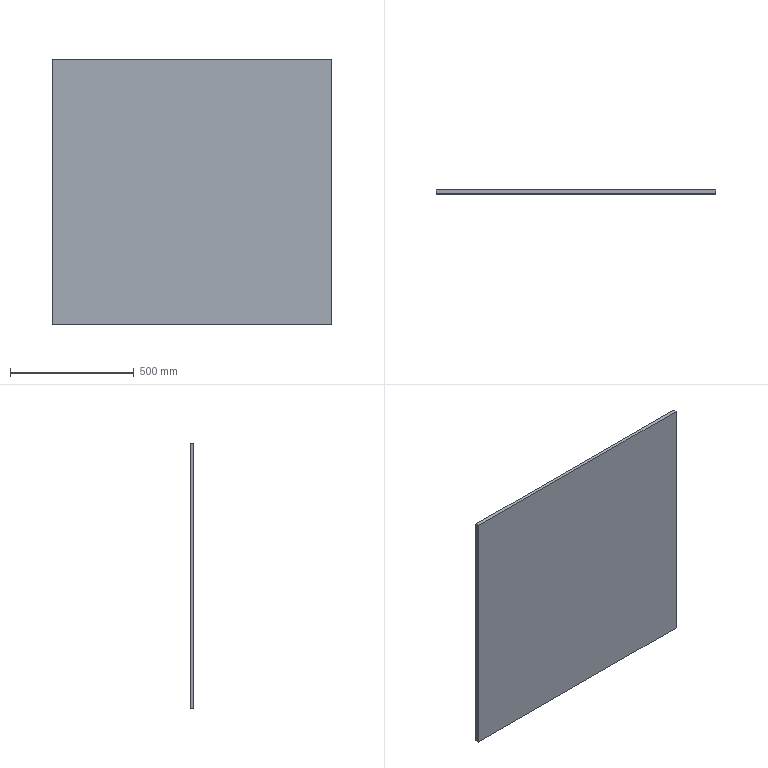Part | SolidWorks | features 3DProfileFeature 1, Extrusion 1, ICE 1 | 1 solid | 6 faces | box 1130 x 15 x 1072 mm | volume 18170400 mm3 | plane 6
STEP:
#1=CARTESIAN_POINT('',(565.,0.,536.));
#2=VERTEX_POINT('',#1);
#3=CARTESIAN_POINT('',(565.,0.,-536.));
#4=VERTEX_POINT('',#3);
#5=CARTESIAN_POINT('',(565.,0.,536.));
#6=DIRECTION('',(0.,0.,-1.));
#7=VECTOR('',#6,1000.);
#8=LINE('',#5,#7);
#9=EDGE_CURVE('',#2,#4,#8,.T.);
#10=ORIENTED_EDGE('',*,*,#9,.T.);
#11=CARTESIAN_POINT('',(565.,15.,-536.));
#12=VERTEX_POINT('',#11);
#13=CARTESIAN_POINT('',(565.,15.,-536.));
#14=DIRECTION('',(0.,-1.,0.));
#15=VECTOR('',#14,1000.);
#16=LINE('',#13,#15);
#17=EDGE_CURVE('',#12,#4,#16,.T.);
#18=ORIENTED_EDGE('',*,*,#17,.F.);
#19=CARTESIAN_POINT('',(565.,15.,536.));
#20=VERTEX_POINT('',#19);
#21=CARTESIAN_POINT('',(565.,15.,536.));
#22=DIRECTION('',(0.,0.,-1.));
#23=VECTOR('',#22,1000.);
#24=LINE('',#21,#23);
#25=EDGE_CURVE('',#20,#12,#24,.T.);
#26=ORIENTED_EDGE('',*,*,#25,.F.);
#27=CARTESIAN_POINT('',(565.,15.,536.));
#28=DIRECTION('',(0.,-1.,0.));
#29=VECTOR('',#28,1000.);
#30=LINE('',#27,#29);
#31=EDGE_CURVE('',#20,#2,#30,.T.);
#32=ORIENTED_EDGE('',*,*,#31,.T.);
#33=EDGE_LOOP('',(#10,#18,#26,#32));
#34=FACE_OUTER_BOUND('',#33,.T.);
#35=CARTESIAN_POINT('',(565.,15.,536.));
#36=DIRECTION('',(-1.,0.,0.));
#37=DIRECTION('',(0.,0.,1.));
#38=AXIS2_PLACEMENT_3D('',#35,#36,#37);
#39=PLANE('',#38);
#40=ADVANCED_FACE('',(#34),#39,.F.);
#41=CARTESIAN_POINT('',(-565.,0.,-536.));
#42=VERTEX_POINT('',#41);
#43=CARTESIAN_POINT('',(-565.,0.,-536.));
#44=DIRECTION('',(-1.,0.,0.));
#45=VECTOR('',#44,1000.);
#46=LINE('',#43,#45);
#47=EDGE_CURVE('',#4,#42,#46,.T.);
#48=ORIENTED_EDGE('',*,*,#47,.T.);
#49=CARTESIAN_POINT('',(-565.,15.,-536.));
#50=VERTEX_POINT('',#49);
#51=CARTESIAN_POINT('',(-565.,15.,-536.));
#52=DIRECTION('',(0.,-1.,0.));
#53=VECTOR('',#52,1000.);
#54=LINE('',#51,#53);
#55=EDGE_CURVE('',#50,#42,#54,.T.);
#56=ORIENTED_EDGE('',*,*,#55,.F.);
#57=CARTESIAN_POINT('',(-565.,15.,-536.));
#58=DIRECTION('',(-1.,0.,0.));
#59=VECTOR('',#58,1000.);
#60=LINE('',#57,#59);
#61=EDGE_CURVE('',#12,#50,#60,.T.);
#62=ORIENTED_EDGE('',*,*,#61,.F.);
#63=ORIENTED_EDGE('',*,*,#17,.T.);
#64=EDGE_LOOP('',(#48,#56,#62,#63));
#65=FACE_OUTER_BOUND('',#64,.T.);
#66=CARTESIAN_POINT('',(-565.,15.,-536.));
#67=DIRECTION('',(0.,0.,1.));
#68=DIRECTION('',(1.,0.,0.));
#69=AXIS2_PLACEMENT_3D('',#66,#67,#68);
#70=PLANE('',#69);
#71=ADVANCED_FACE('',(#65),#70,.F.);
#72=CARTESIAN_POINT('',(-565.,0.,536.));
#73=VERTEX_POINT('',#72);
#74=CARTESIAN_POINT('',(-565.,0.,536.));
#75=DIRECTION('',(0.,0.,1.));
#76=VECTOR('',#75,1000.);
#77=LINE('',#74,#76);
#78=EDGE_CURVE('',#42,#73,#77,.T.);
#79=ORIENTED_EDGE('',*,*,#78,.T.);
#80=CARTESIAN_POINT('',(-565.,15.,536.));
#81=VERTEX_POINT('',#80);
#82=CARTESIAN_POINT('',(-565.,15.,536.));
#83=DIRECTION('',(0.,-1.,0.));
#84=VECTOR('',#83,1000.);
#85=LINE('',#82,#84);
#86=EDGE_CURVE('',#81,#73,#85,.T.);
#87=ORIENTED_EDGE('',*,*,#86,.F.);
#88=CARTESIAN_POINT('',(-565.,15.,536.));
#89=DIRECTION('',(0.,0.,1.));
#90=VECTOR('',#89,1000.);
#91=LINE('',#88,#90);
#92=EDGE_CURVE('',#50,#81,#91,.T.);
#93=ORIENTED_EDGE('',*,*,#92,.F.);
#94=ORIENTED_EDGE('',*,*,#55,.T.);
#95=EDGE_LOOP('',(#79,#87,#93,#94));
#96=FACE_OUTER_BOUND('',#95,.T.);
#97=CARTESIAN_POINT('',(-565.,15.,536.));
#98=DIRECTION('',(1.,0.,0.));
#99=DIRECTION('',(0.,0.,-1.));
#100=AXIS2_PLACEMENT_3D('',#97,#98,#99);
#101=PLANE('',#100);
#102=ADVANCED_FACE('',(#96),#101,.F.);
#103=CARTESIAN_POINT('',(-565.,0.,536.));
#104=DIRECTION('',(1.,0.,0.));
#105=VECTOR('',#104,1000.);
#106=LINE('',#103,#105);
#107=EDGE_CURVE('',#73,#2,#106,.T.);
#108=ORIENTED_EDGE('',*,*,#107,.T.);
#109=ORIENTED_EDGE('',*,*,#31,.F.);
#110=CARTESIAN_POINT('',(-565.,15.,536.));
#111=DIRECTION('',(1.,0.,0.));
#112=VECTOR('',#111,1000.);
#113=LINE('',#110,#112);
#114=EDGE_CURVE('',#81,#20,#113,.T.);
#115=ORIENTED_EDGE('',*,*,#114,.F.);
#116=ORIENTED_EDGE('',*,*,#86,.T.);
#117=EDGE_LOOP('',(#108,#109,#115,#116));
#118=FACE_OUTER_BOUND('',#117,.T.);
#119=CARTESIAN_POINT('',(-565.,15.,536.));
#120=DIRECTION('',(0.,0.,-1.));
#121=DIRECTION('',(-1.,0.,0.));
#122=AXIS2_PLACEMENT_3D('',#119,#120,#121);
#123=PLANE('',#122);
#124=ADVANCED_FACE('',(#118),#123,.F.);
#125=ORIENTED_EDGE('',*,*,#25,.T.);
#126=ORIENTED_EDGE('',*,*,#61,.T.);
#127=ORIENTED_EDGE('',*,*,#92,.T.);
#128=ORIENTED_EDGE('',*,*,#114,.T.);
#129=EDGE_LOOP('',(#125,#126,#127,#128));
#130=FACE_OUTER_BOUND('',#129,.T.);
#131=CARTESIAN_POINT('',(0.,15.,0.));
#132=DIRECTION('',(0.,-1.,0.));
#133=DIRECTION('',(0.,0.,-1.));
#134=AXIS2_PLACEMENT_3D('',#131,#132,#133);
#135=PLANE('',#134);
#136=ADVANCED_FACE('',(#130),#135,.F.);
#137=ORIENTED_EDGE('',*,*,#9,.F.);
#138=ORIENTED_EDGE('',*,*,#107,.F.);
#139=ORIENTED_EDGE('',*,*,#78,.F.);
#140=ORIENTED_EDGE('',*,*,#47,.F.);
#141=EDGE_LOOP('',(#137,#138,#139,#140));
#142=FACE_OUTER_BOUND('',#141,.T.);
#143=CARTESIAN_POINT('',(0.,0.,0.));
#144=DIRECTION('',(0.,-1.,0.));
#145=DIRECTION('',(0.,0.,-1.));
#146=AXIS2_PLACEMENT_3D('',#143,#144,#145);
#147=PLANE('',#146);
#148=ADVANCED_FACE('',(#142),#147,.T.);
#149=CLOSED_SHELL('',(#40,#71,#102,#124,#136,#148));
#150=MANIFOLD_SOLID_BREP('',#149);
#151=CARTESIAN_POINT('',(0.,0.,0.));
#152=DIRECTION('',(0.,0.,1.));
#153=DIRECTION('',(1.,0.,0.));
#154=AXIS2_PLACEMENT_3D('',#151,#152,#153);
#155=(LENGTH_UNIT()NAMED_UNIT(*)SI_UNIT(.MILLI.,.METRE.));
#156=UNCERTAINTY_MEASURE_WITH_UNIT(LENGTH_MEASURE(0.00001),#155,'','');
#157=(NAMED_UNIT(*)PLANE_ANGLE_UNIT()SI_UNIT($,.RADIAN.));
#158=(NAMED_UNIT(*)SI_UNIT($,.STERADIAN.)SOLID_ANGLE_UNIT());
#159=(GEOMETRIC_REPRESENTATION_CONTEXT(3)GLOBAL_UNCERTAINTY_ASSIGNED_CONTEXT((#156))GLOBAL_UNIT_ASSIGNED_CONTEXT((#155,#157,#158))REPRESENTATION_CONTEXT('',''));
#160=ADVANCED_BREP_SHAPE_REPRESENTATION('',(#150,#154),#159);